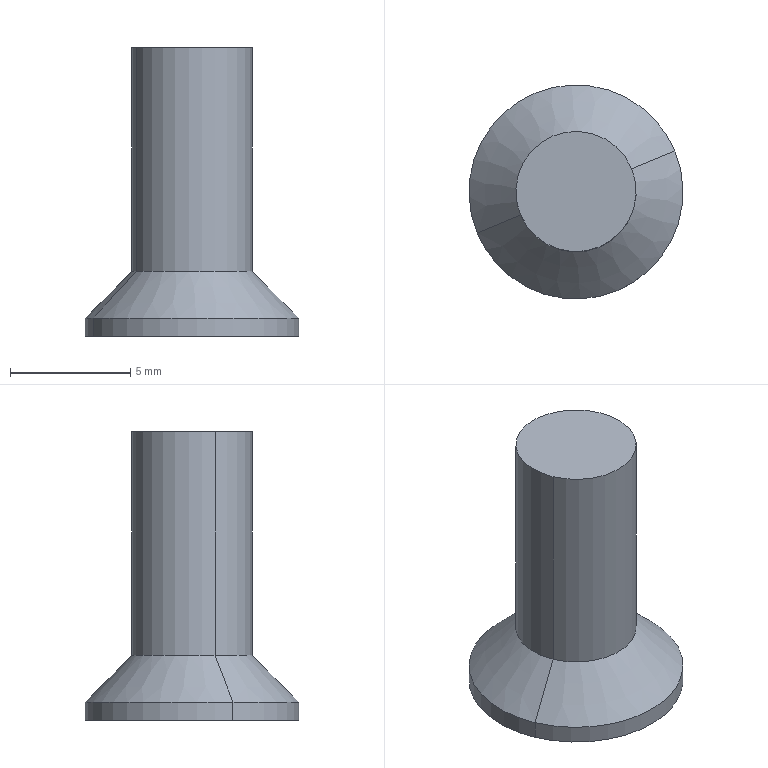Part | SolidWorks | features SplitBody 1 | 1 solid | 41 faces | box 8.9 x 8.9 x 12 mm | volume 292.842 mm3 | plane 31 | cylinder 8 | cone 2 | commonest cylinder face diameters 0.6 x4 5 x2 8.9 x2
STEP:
#1=CARTESIAN_POINT('',(595.745,101.287,-497.016));
#2=VERTEX_POINT('',#1);
#3=CARTESIAN_POINT('',(591.126,99.372,-497.016));
#4=VERTEX_POINT('',#3);
#5=CARTESIAN_POINT('',(593.436,100.329,-497.016));
#6=DIRECTION('',(0.,0.,1.));
#7=DIRECTION('',(0.9237,0.383,0.));
#8=AXIS2_PLACEMENT_3D('',#5,#6,#7);
#9=CIRCLE('',#8,2.5);
#10=EDGE_CURVE('',#2,#4,#9,.T.);
#11=ORIENTED_EDGE('',*,*,#10,.T.);
#12=CARTESIAN_POINT('',(591.126,99.372,-487.716));
#13=VERTEX_POINT('',#12);
#14=CARTESIAN_POINT('',(591.126,99.372,-495.2));
#15=DIRECTION('',(0.,0.,1.));
#16=VECTOR('',#15,1000.);
#17=LINE('',#14,#16);
#18=EDGE_CURVE('',#4,#13,#17,.T.);
#19=ORIENTED_EDGE('',*,*,#18,.T.);
#20=CARTESIAN_POINT('',(595.745,101.287,-487.716));
#21=VERTEX_POINT('',#20);
#22=CARTESIAN_POINT('',(593.436,100.329,-487.716));
#23=DIRECTION('',(0.,0.,1.));
#24=DIRECTION('',(0.9237,0.383,0.));
#25=AXIS2_PLACEMENT_3D('',#22,#23,#24);
#26=CIRCLE('',#25,2.5);
#27=EDGE_CURVE('',#21,#13,#26,.T.);
#28=ORIENTED_EDGE('',*,*,#27,.F.);
#29=CARTESIAN_POINT('',(595.745,101.287,-495.2));
#30=DIRECTION('',(0.,0.,1.));
#31=VECTOR('',#30,1000.);
#32=LINE('',#29,#31);
#33=EDGE_CURVE('',#2,#21,#32,.T.);
#34=ORIENTED_EDGE('',*,*,#33,.F.);
#35=EDGE_LOOP('',(#11,#19,#28,#34));
#36=FACE_OUTER_BOUND('',#35,.T.);
#37=CARTESIAN_POINT('',(593.436,100.329,-495.2));
#38=DIRECTION('',(0.,0.,1.));
#39=DIRECTION('',(0.9237,0.383,0.));
#40=AXIS2_PLACEMENT_3D('',#37,#38,#39);
#41=CYLINDRICAL_SURFACE('',#40,2.5);
#42=ADVANCED_FACE('',(#36),#41,.T.);
#43=ORIENTED_EDGE('',*,*,#10,.F.);
#44=CARTESIAN_POINT('',(597.546,102.034,-498.966));
#45=VERTEX_POINT('',#44);
#46=CARTESIAN_POINT('',(595.745,101.287,-497.016));
#47=DIRECTION('',(0.6532,0.2709,-0.7071));
#48=VECTOR('',#47,1000.);
#49=LINE('',#46,#48);
#50=EDGE_CURVE('',#2,#45,#49,.T.);
#51=ORIENTED_EDGE('',*,*,#50,.T.);
#52=CARTESIAN_POINT('',(589.325,98.625,-498.966));
#53=VERTEX_POINT('',#52);
#54=CARTESIAN_POINT('',(593.436,100.329,-498.966));
#55=DIRECTION('',(0.,0.,1.));
#56=DIRECTION('',(0.9237,0.383,0.));
#57=AXIS2_PLACEMENT_3D('',#54,#55,#56);
#58=CIRCLE('',#57,4.45);
#59=EDGE_CURVE('',#45,#53,#58,.T.);
#60=ORIENTED_EDGE('',*,*,#59,.T.);
#61=CARTESIAN_POINT('',(591.126,99.372,-497.016));
#62=DIRECTION('',(-0.6532,-0.2709,-0.7071));
#63=VECTOR('',#62,1000.);
#64=LINE('',#61,#63);
#65=EDGE_CURVE('',#4,#53,#64,.T.);
#66=ORIENTED_EDGE('',*,*,#65,.F.);
#67=EDGE_LOOP('',(#43,#51,#60,#66));
#68=FACE_OUTER_BOUND('',#67,.T.);
#69=CARTESIAN_POINT('',(593.436,100.329,-497.016));
#70=DIRECTION('',(0.,0.,-1.));
#71=DIRECTION('',(-0.9237,-0.383,0.));
#72=AXIS2_PLACEMENT_3D('',#69,#70,#71);
#73=CONICAL_SURFACE('',#72,2.5,0.7854);
#74=ADVANCED_FACE('',(#68),#73,.T.);
#75=CARTESIAN_POINT('',(597.546,102.034,-499.716));
#76=VERTEX_POINT('',#75);
#77=CARTESIAN_POINT('',(589.325,98.625,-499.716));
#78=VERTEX_POINT('',#77);
#79=CARTESIAN_POINT('',(593.436,100.329,-499.716));
#80=DIRECTION('',(0.,0.,1.));
#81=DIRECTION('',(0.9237,0.383,0.));
#82=AXIS2_PLACEMENT_3D('',#79,#80,#81);
#83=CIRCLE('',#82,4.45);
#84=EDGE_CURVE('',#76,#78,#83,.T.);
#85=ORIENTED_EDGE('',*,*,#84,.T.);
#86=CARTESIAN_POINT('',(589.325,98.625,-495.2));
#87=DIRECTION('',(0.,0.,1.));
#88=VECTOR('',#87,1000.);
#89=LINE('',#86,#88);
#90=EDGE_CURVE('',#78,#53,#89,.T.);
#91=ORIENTED_EDGE('',*,*,#90,.T.);
#92=ORIENTED_EDGE('',*,*,#59,.F.);
#93=CARTESIAN_POINT('',(597.546,102.034,-495.2));
#94=DIRECTION('',(0.,0.,1.));
#95=VECTOR('',#94,1000.);
#96=LINE('',#93,#95);
#97=EDGE_CURVE('',#76,#45,#96,.T.);
#98=ORIENTED_EDGE('',*,*,#97,.F.);
#99=EDGE_LOOP('',(#85,#91,#92,#98));
#100=FACE_OUTER_BOUND('',#99,.T.);
#101=CARTESIAN_POINT('',(593.436,100.329,-495.2));
#102=DIRECTION('',(0.,0.,1.));
#103=DIRECTION('',(0.9237,0.383,0.));
#104=AXIS2_PLACEMENT_3D('',#101,#102,#103);
#105=CYLINDRICAL_SURFACE('',#104,4.45);
#106=ADVANCED_FACE('',(#100),#105,.T.);
#107=ORIENTED_EDGE('',*,*,#84,.F.);
#108=CARTESIAN_POINT('',(593.436,100.329,-499.716));
#109=DIRECTION('',(0.,0.,1.));
#110=DIRECTION('',(0.9237,0.383,0.));
#111=AXIS2_PLACEMENT_3D('',#108,#109,#110);
#112=CIRCLE('',#111,4.45);
#113=EDGE_CURVE('',#78,#76,#112,.T.);
#114=ORIENTED_EDGE('',*,*,#113,.F.);
#115=EDGE_LOOP('',(#107,#114));
#116=FACE_OUTER_BOUND('',#115,.T.);
#117=CARTESIAN_POINT('',(595.638,101.806,-499.716));
#118=VERTEX_POINT('',#117);
#119=CARTESIAN_POINT('',(594.232,101.222,-499.716));
#120=VERTEX_POINT('',#119);
#121=CARTESIAN_POINT('',(593.717,101.009,-499.716));
#122=DIRECTION('',(-0.9237,-0.383,0.));
#123=VECTOR('',#122,1000.);
#124=LINE('',#121,#123);
#125=EDGE_CURVE('',#118,#120,#124,.T.);
#126=ORIENTED_EDGE('',*,*,#125,.T.);
#127=CARTESIAN_POINT('',(594.43,102.732,-499.716));
#128=VERTEX_POINT('',#127);
#129=CARTESIAN_POINT('',(594.153,100.627,-499.716));
#130=DIRECTION('',(0.1301,0.9915,0.));
#131=VECTOR('',#130,1000.);
#132=LINE('',#129,#131);
#133=EDGE_CURVE('',#120,#128,#132,.T.);
#134=ORIENTED_EDGE('',*,*,#133,.T.);
#135=CARTESIAN_POINT('',(593.503,101.524,-499.716));
#136=VERTEX_POINT('',#135);
#137=CARTESIAN_POINT('',(593.138,101.047,-499.716));
#138=DIRECTION('',(-0.6084,-0.7936,0.));
#139=VECTOR('',#138,1000.);
#140=LINE('',#137,#139);
#141=EDGE_CURVE('',#128,#136,#140,.T.);
#142=ORIENTED_EDGE('',*,*,#141,.T.);
#143=CARTESIAN_POINT('',(592.92,102.93,-499.716));
#144=VERTEX_POINT('',#143);
#145=CARTESIAN_POINT('',(593.717,101.009,-499.716));
#146=DIRECTION('',(-0.383,0.9237,0.));
#147=VECTOR('',#146,1000.);
#148=LINE('',#145,#147);
#149=EDGE_CURVE('',#136,#144,#148,.T.);
#150=ORIENTED_EDGE('',*,*,#149,.T.);
#151=CARTESIAN_POINT('',(591.959,102.532,-499.716));
#152=VERTEX_POINT('',#151);
#153=CARTESIAN_POINT('',(592.92,102.93,-499.716));
#154=DIRECTION('',(-0.9237,-0.383,0.));
#155=VECTOR('',#154,1000.);
#156=LINE('',#153,#155);
#157=EDGE_CURVE('',#144,#152,#156,.T.);
#158=ORIENTED_EDGE('',*,*,#157,.T.);
#159=CARTESIAN_POINT('',(592.543,101.125,-499.716));
#160=VERTEX_POINT('',#159);
#161=CARTESIAN_POINT('',(592.756,100.611,-499.716));
#162=DIRECTION('',(0.383,-0.9237,0.));
#163=VECTOR('',#162,1000.);
#164=LINE('',#161,#163);
#165=EDGE_CURVE('',#152,#160,#164,.T.);
#166=ORIENTED_EDGE('',*,*,#165,.T.);
#167=CARTESIAN_POINT('',(591.033,101.323,-499.716));
#168=VERTEX_POINT('',#167);
#169=CARTESIAN_POINT('',(593.138,101.047,-499.716));
#170=DIRECTION('',(-0.9915,0.1301,0.));
#171=VECTOR('',#170,1000.);
#172=LINE('',#169,#171);
#173=EDGE_CURVE('',#160,#168,#172,.T.);
#174=ORIENTED_EDGE('',*,*,#173,.T.);
#175=CARTESIAN_POINT('',(592.241,100.397,-499.716));
#176=VERTEX_POINT('',#175);
#177=CARTESIAN_POINT('',(592.718,100.032,-499.716));
#178=DIRECTION('',(0.7936,-0.6084,0.));
#179=VECTOR('',#178,1000.);
#180=LINE('',#177,#179);
#181=EDGE_CURVE('',#168,#176,#180,.T.);
#182=ORIENTED_EDGE('',*,*,#181,.T.);
#183=CARTESIAN_POINT('',(590.835,99.814,-499.716));
#184=VERTEX_POINT('',#183);
#185=CARTESIAN_POINT('',(592.756,100.611,-499.716));
#186=DIRECTION('',(-0.9237,-0.383,0.));
#187=VECTOR('',#186,1000.);
#188=LINE('',#185,#187);
#189=EDGE_CURVE('',#176,#184,#188,.T.);
#190=ORIENTED_EDGE('',*,*,#189,.T.);
#191=CARTESIAN_POINT('',(591.233,98.853,-499.716));
#192=VERTEX_POINT('',#191);
#193=CARTESIAN_POINT('',(590.835,99.814,-499.716));
#194=DIRECTION('',(0.383,-0.9237,0.));
#195=VECTOR('',#194,1000.);
#196=LINE('',#193,#195);
#197=EDGE_CURVE('',#184,#192,#196,.T.);
#198=ORIENTED_EDGE('',*,*,#197,.T.);
#199=CARTESIAN_POINT('',(592.64,99.436,-499.716));
#200=VERTEX_POINT('',#199);
#201=CARTESIAN_POINT('',(593.155,99.65,-499.716));
#202=DIRECTION('',(0.9237,0.383,0.));
#203=VECTOR('',#202,1000.);
#204=LINE('',#201,#203);
#205=EDGE_CURVE('',#192,#200,#204,.T.);
#206=ORIENTED_EDGE('',*,*,#205,.T.);
#207=CARTESIAN_POINT('',(592.442,97.927,-499.716));
#208=VERTEX_POINT('',#207);
#209=CARTESIAN_POINT('',(592.718,100.032,-499.716));
#210=DIRECTION('',(-0.1301,-0.9915,0.));
#211=VECTOR('',#210,1000.);
#212=LINE('',#209,#211);
#213=EDGE_CURVE('',#200,#208,#212,.T.);
#214=ORIENTED_EDGE('',*,*,#213,.T.);
#215=CARTESIAN_POINT('',(593.368,99.135,-499.716));
#216=VERTEX_POINT('',#215);
#217=CARTESIAN_POINT('',(593.733,99.612,-499.716));
#218=DIRECTION('',(0.6084,0.7936,0.));
#219=VECTOR('',#218,1000.);
#220=LINE('',#217,#219);
#221=EDGE_CURVE('',#208,#216,#220,.T.);
#222=ORIENTED_EDGE('',*,*,#221,.T.);
#223=CARTESIAN_POINT('',(593.951,97.728,-499.716));
#224=VERTEX_POINT('',#223);
#225=CARTESIAN_POINT('',(593.155,99.65,-499.716));
#226=DIRECTION('',(0.383,-0.9237,0.));
#227=VECTOR('',#226,1000.);
#228=LINE('',#225,#227);
#229=EDGE_CURVE('',#216,#224,#228,.T.);
#230=ORIENTED_EDGE('',*,*,#229,.T.);
#231=CARTESIAN_POINT('',(594.912,98.127,-499.716));
#232=VERTEX_POINT('',#231);
#233=CARTESIAN_POINT('',(594.912,98.127,-499.716));
#234=DIRECTION('',(0.9237,0.383,0.));
#235=VECTOR('',#234,1000.);
#236=LINE('',#233,#235);
#237=EDGE_CURVE('',#224,#232,#236,.T.);
#238=ORIENTED_EDGE('',*,*,#237,.T.);
#239=CARTESIAN_POINT('',(594.329,99.533,-499.716));
#240=VERTEX_POINT('',#239);
#241=CARTESIAN_POINT('',(594.115,100.048,-499.716));
#242=DIRECTION('',(-0.383,0.9237,0.));
#243=VECTOR('',#242,1000.);
#244=LINE('',#241,#243);
#245=EDGE_CURVE('',#232,#240,#244,.T.);
#246=ORIENTED_EDGE('',*,*,#245,.T.);
#247=CARTESIAN_POINT('',(595.838,99.335,-499.716));
#248=VERTEX_POINT('',#247);
#249=CARTESIAN_POINT('',(593.733,99.612,-499.716));
#250=DIRECTION('',(0.9915,-0.1301,0.));
#251=VECTOR('',#250,1000.);
#252=LINE('',#249,#251);
#253=EDGE_CURVE('',#240,#248,#252,.T.);
#254=ORIENTED_EDGE('',*,*,#253,.T.);
#255=CARTESIAN_POINT('',(594.63,100.262,-499.716));
#256=VERTEX_POINT('',#255);
#257=CARTESIAN_POINT('',(594.153,100.627,-499.716));
#258=DIRECTION('',(-0.7936,0.6084,0.));
#259=VECTOR('',#258,1000.);
#260=LINE('',#257,#259);
#261=EDGE_CURVE('',#248,#256,#260,.T.);
#262=ORIENTED_EDGE('',*,*,#261,.T.);
#263=CARTESIAN_POINT('',(596.037,100.845,-499.716));
#264=VERTEX_POINT('',#263);
#265=CARTESIAN_POINT('',(594.115,100.048,-499.716));
#266=DIRECTION('',(0.9237,0.383,0.));
#267=VECTOR('',#266,1000.);
#268=LINE('',#265,#267);
#269=EDGE_CURVE('',#256,#264,#268,.T.);
#270=ORIENTED_EDGE('',*,*,#269,.T.);
#271=CARTESIAN_POINT('',(595.638,101.806,-499.716));
#272=DIRECTION('',(-0.383,0.9237,0.));
#273=VECTOR('',#272,1000.);
#274=LINE('',#271,#273);
#275=EDGE_CURVE('',#264,#118,#274,.T.);
#276=ORIENTED_EDGE('',*,*,#275,.T.);
#277=EDGE_LOOP('',(#126,#134,#142,#150,#158,#166,#174,#182,#190,#198,#206,#214,#222,#230,#238,#246,#254,#262,#270,#276));
#278=FACE_BOUND('',#277,.T.);
#279=CARTESIAN_POINT('',(591.731,104.44,-499.716));
#280=DIRECTION('',(0.,0.,-1.));
#281=DIRECTION('',(-0.9237,-0.383,0.));
#282=AXIS2_PLACEMENT_3D('',#279,#280,#281);
#283=PLANE('',#282);
#284=ADVANCED_FACE('',(#116,#278),#283,.T.);
#285=ORIENTED_EDGE('',*,*,#189,.F.);
#286=CARTESIAN_POINT('',(592.479,100.496,-499.104));
#287=VERTEX_POINT('',#286);
#288=CARTESIAN_POINT('',(592.764,100.614,-498.37));
#289=DIRECTION('',(0.3579,0.1484,0.9219));
#290=VECTOR('',#289,1000.);
#291=LINE('',#288,#290);
#292=EDGE_CURVE('',#176,#287,#291,.T.);
#293=ORIENTED_EDGE('',*,*,#292,.T.);
#294=CARTESIAN_POINT('',(592.479,100.496,-498.366));
#295=VERTEX_POINT('',#294);
#296=CARTESIAN_POINT('',(592.479,100.496,-498.366));
#297=DIRECTION('',(0.,0.,1.));
#298=VECTOR('',#297,1000.);
#299=LINE('',#296,#298);
#300=EDGE_CURVE('',#287,#295,#299,.T.);
#301=ORIENTED_EDGE('',*,*,#300,.T.);
#302=CARTESIAN_POINT('',(591.555,100.112,-498.366));
#303=VERTEX_POINT('',#302);
#304=CARTESIAN_POINT('',(592.756,100.611,-498.366));
#305=DIRECTION('',(-0.9237,-0.383,0.));
#306=VECTOR('',#305,1000.);
#307=LINE('',#304,#306);
#308=EDGE_CURVE('',#295,#303,#307,.T.);
#309=ORIENTED_EDGE('',*,*,#308,.T.);
#310=CARTESIAN_POINT('',(590.835,99.814,-499.716));
#311=DIRECTION('',(-0.4619,-0.1915,-0.866));
#312=VECTOR('',#311,1000.);
#313=LINE('',#310,#312);
#314=EDGE_CURVE('',#303,#184,#313,.T.);
#315=ORIENTED_EDGE('',*,*,#314,.T.);
#316=EDGE_LOOP('',(#285,#293,#301,#309,#315));
#317=FACE_OUTER_BOUND('',#316,.T.);
#318=CARTESIAN_POINT('',(592.756,100.611,-498.366));
#319=DIRECTION('',(0.383,-0.9237,0.));
#320=DIRECTION('',(0.9237,0.383,0.));
#321=AXIS2_PLACEMENT_3D('',#318,#319,#320);
#322=PLANE('',#321);
#323=ADVANCED_FACE('',(#317),#322,.T.);
#324=CARTESIAN_POINT('',(592.877,99.535,-498.366));
#325=VERTEX_POINT('',#324);
#326=CARTESIAN_POINT('',(592.877,99.535,-499.104));
#327=VERTEX_POINT('',#326);
#328=CARTESIAN_POINT('',(592.877,99.535,-498.366));
#329=DIRECTION('',(0.,0.,-1.));
#330=VECTOR('',#329,1000.);
#331=LINE('',#328,#330);
#332=EDGE_CURVE('',#325,#327,#331,.T.);
#333=ORIENTED_EDGE('',*,*,#332,.T.);
#334=CARTESIAN_POINT('',(593.162,99.653,-498.37));
#335=DIRECTION('',(-0.3579,-0.1484,-0.9219));
#336=VECTOR('',#335,1000.);
#337=LINE('',#334,#336);
#338=EDGE_CURVE('',#327,#200,#337,.T.);
#339=ORIENTED_EDGE('',*,*,#338,.T.);
#340=ORIENTED_EDGE('',*,*,#205,.F.);
#341=CARTESIAN_POINT('',(591.953,99.152,-498.366));
#342=VERTEX_POINT('',#341);
#343=CARTESIAN_POINT('',(592.254,99.276,-497.803));
#344=DIRECTION('',(-0.4619,-0.1915,-0.866));
#345=VECTOR('',#344,1000.);
#346=LINE('',#343,#345);
#347=EDGE_CURVE('',#342,#192,#346,.T.);
#348=ORIENTED_EDGE('',*,*,#347,.F.);
#349=CARTESIAN_POINT('',(593.155,99.65,-498.366));
#350=DIRECTION('',(0.9237,0.383,0.));
#351=VECTOR('',#350,1000.);
#352=LINE('',#349,#351);
#353=EDGE_CURVE('',#342,#325,#352,.T.);
#354=ORIENTED_EDGE('',*,*,#353,.T.);
#355=EDGE_LOOP('',(#333,#339,#340,#348,#354));
#356=FACE_OUTER_BOUND('',#355,.T.);
#357=CARTESIAN_POINT('',(593.155,99.65,-498.366));
#358=DIRECTION('',(-0.383,0.9237,0.));
#359=DIRECTION('',(-0.9237,-0.383,0.));
#360=AXIS2_PLACEMENT_3D('',#357,#358,#359);
#361=PLANE('',#360);
#362=ADVANCED_FACE('',(#356),#361,.T.);
#363=ORIENTED_EDGE('',*,*,#229,.F.);
#364=CARTESIAN_POINT('',(593.269,99.373,-499.104));
#365=VERTEX_POINT('',#364);
#366=CARTESIAN_POINT('',(593.151,99.658,-498.37));
#367=DIRECTION('',(-0.1484,0.3579,0.9219));
#368=VECTOR('',#367,1000.);
#369=LINE('',#366,#368);
#370=EDGE_CURVE('',#216,#365,#369,.T.);
#371=ORIENTED_EDGE('',*,*,#370,.T.);
#372=CARTESIAN_POINT('',(593.269,99.373,-498.366));
#373=VERTEX_POINT('',#372);
#374=CARTESIAN_POINT('',(593.269,99.373,-498.366));
#375=DIRECTION('',(0.,0.,1.));
#376=VECTOR('',#375,1000.);
#377=LINE('',#374,#376);
#378=EDGE_CURVE('',#365,#373,#377,.T.);
#379=ORIENTED_EDGE('',*,*,#378,.T.);
#380=CARTESIAN_POINT('',(593.653,98.448,-498.366));
#381=VERTEX_POINT('',#380);
#382=CARTESIAN_POINT('',(593.155,99.65,-498.366));
#383=DIRECTION('',(0.383,-0.9237,0.));
#384=VECTOR('',#383,1000.);
#385=LINE('',#382,#384);
#386=EDGE_CURVE('',#373,#381,#385,.T.);
#387=ORIENTED_EDGE('',*,*,#386,.T.);
#388=CARTESIAN_POINT('',(593.951,97.728,-499.716));
#389=DIRECTION('',(0.1915,-0.4619,-0.866));
#390=VECTOR('',#389,1000.);
#391=LINE('',#388,#390);
#392=EDGE_CURVE('',#381,#224,#391,.T.);
#393=ORIENTED_EDGE('',*,*,#392,.T.);
#394=EDGE_LOOP('',(#363,#371,#379,#387,#393));
#395=FACE_OUTER_BOUND('',#394,.T.);
#396=CARTESIAN_POINT('',(593.155,99.65,-498.366));
#397=DIRECTION('',(0.9237,0.383,0.));
#398=DIRECTION('',(-0.383,0.9237,0.));
#399=AXIS2_PLACEMENT_3D('',#396,#397,#398);
#400=PLANE('',#399);
#401=ADVANCED_FACE('',(#395),#400,.T.);
#402=CARTESIAN_POINT('',(594.23,99.771,-498.366));
#403=VERTEX_POINT('',#402);
#404=CARTESIAN_POINT('',(594.23,99.771,-499.104));
#405=VERTEX_POINT('',#404);
#406=CARTESIAN_POINT('',(594.23,99.771,-498.366));
#407=DIRECTION('',(0.,0.,-1.));
#408=VECTOR('',#407,1000.);
#409=LINE('',#406,#408);
#410=EDGE_CURVE('',#403,#405,#409,.T.);
#411=ORIENTED_EDGE('',*,*,#410,.T.);
#412=CARTESIAN_POINT('',(594.112,100.056,-498.37));
#413=DIRECTION('',(0.1484,-0.3579,-0.9219));
#414=VECTOR('',#413,1000.);
#415=LINE('',#412,#414);
#416=EDGE_CURVE('',#405,#240,#415,.T.);
#417=ORIENTED_EDGE('',*,*,#416,.T.);
#418=ORIENTED_EDGE('',*,*,#245,.F.);
#419=CARTESIAN_POINT('',(594.613,98.847,-498.366));
#420=VERTEX_POINT('',#419);
#421=CARTESIAN_POINT('',(594.489,99.147,-497.803));
#422=DIRECTION('',(0.1915,-0.4619,-0.866));
#423=VECTOR('',#422,1000.);
#424=LINE('',#421,#423);
#425=EDGE_CURVE('',#420,#232,#424,.T.);
#426=ORIENTED_EDGE('',*,*,#425,.F.);
#427=CARTESIAN_POINT('',(594.115,100.048,-498.366));
#428=DIRECTION('',(-0.383,0.9237,0.));
#429=VECTOR('',#428,1000.);
#430=LINE('',#427,#429);
#431=EDGE_CURVE('',#420,#403,#430,.T.);
#432=ORIENTED_EDGE('',*,*,#431,.T.);
#433=EDGE_LOOP('',(#411,#417,#418,#426,#432));
#434=FACE_OUTER_BOUND('',#433,.T.);
#435=CARTESIAN_POINT('',(594.115,100.048,-498.366));
#436=DIRECTION('',(-0.9237,-0.383,0.));
#437=DIRECTION('',(0.,0.,1.));
#438=AXIS2_PLACEMENT_3D('',#435,#436,#437);
#439=PLANE('',#438);
#440=ADVANCED_FACE('',(#434),#439,.T.);
#441=ORIENTED_EDGE('',*,*,#269,.F.);
#442=CARTESIAN_POINT('',(594.392,100.163,-499.104));
#443=VERTEX_POINT('',#442);
#444=CARTESIAN_POINT('',(594.107,100.045,-498.37));
#445=DIRECTION('',(-0.3579,-0.1484,0.9219));
#446=VECTOR('',#445,1000.);
#447=LINE('',#444,#446);
#448=EDGE_CURVE('',#256,#443,#447,.T.);
#449=ORIENTED_EDGE('',*,*,#448,.T.);
#450=CARTESIAN_POINT('',(594.392,100.163,-498.366));
#451=VERTEX_POINT('',#450);
#452=CARTESIAN_POINT('',(594.392,100.163,-498.366));
#453=DIRECTION('',(0.,0.,1.));
#454=VECTOR('',#453,1000.);
#455=LINE('',#452,#454);
#456=EDGE_CURVE('',#443,#451,#455,.T.);
#457=ORIENTED_EDGE('',*,*,#456,.T.);
#458=CARTESIAN_POINT('',(595.317,100.546,-498.366));
#459=VERTEX_POINT('',#458);
#460=CARTESIAN_POINT('',(594.115,100.048,-498.366));
#461=DIRECTION('',(0.9237,0.383,0.));
#462=VECTOR('',#461,1000.);
#463=LINE('',#460,#462);
#464=EDGE_CURVE('',#451,#459,#463,.T.);
#465=ORIENTED_EDGE('',*,*,#464,.T.);
#466=CARTESIAN_POINT('',(596.037,100.845,-499.716));
#467=DIRECTION('',(0.4619,0.1915,-0.866));
#468=VECTOR('',#467,1000.);
#469=LINE('',#466,#468);
#470=EDGE_CURVE('',#459,#264,#469,.T.);
#471=ORIENTED_EDGE('',*,*,#470,.T.);
#472=EDGE_LOOP('',(#441,#449,#457,#465,#471));
#473=FACE_OUTER_BOUND('',#472,.T.);
#474=CARTESIAN_POINT('',(594.115,100.048,-498.366));
#475=DIRECTION('',(-0.383,0.9237,0.));
#476=DIRECTION('',(-0.9237,-0.383,0.));
#477=AXIS2_PLACEMENT_3D('',#474,#475,#476);
#478=PLANE('',#477);
#479=ADVANCED_FACE('',(#473),#478,.T.);
#480=CARTESIAN_POINT('',(593.994,101.124,-498.366));
#481=VERTEX_POINT('',#480);
#482=CARTESIAN_POINT('',(593.994,101.124,-499.104));
#483=VERTEX_POINT('',#482);
#484=CARTESIAN_POINT('',(593.994,101.124,-498.366));
#485=DIRECTION('',(0.,0.,-1.));
#486=VECTOR('',#485,1000.);
#487=LINE('',#484,#486);
#488=EDGE_CURVE('',#481,#483,#487,.T.);
#489=ORIENTED_EDGE('',*,*,#488,.T.);
#490=CARTESIAN_POINT('',(593.709,101.006,-498.37));
#491=DIRECTION('',(0.3579,0.1484,-0.9219));
#492=VECTOR('',#491,1000.);
#493=LINE('',#490,#492);
#494=EDGE_CURVE('',#483,#120,#493,.T.);
#495=ORIENTED_EDGE('',*,*,#494,.T.);
#496=ORIENTED_EDGE('',*,*,#125,.F.);
#497=CARTESIAN_POINT('',(594.918,101.507,-498.366));
#498=VERTEX_POINT('',#497);
#499=CARTESIAN_POINT('',(594.618,101.383,-497.803));
#500=DIRECTION('',(0.4619,0.1915,-0.866));
#501=VECTOR('',#500,1000.);
#502=LINE('',#499,#501);
#503=EDGE_CURVE('',#498,#118,#502,.T.);
#504=ORIENTED_EDGE('',*,*,#503,.F.);
#505=CARTESIAN_POINT('',(593.717,101.009,-498.366));
#506=DIRECTION('',(-0.9237,-0.383,0.));
#507=VECTOR('',#506,1000.);
#508=LINE('',#505,#507);
#509=EDGE_CURVE('',#498,#481,#508,.T.);
#510=ORIENTED_EDGE('',*,*,#509,.T.);
#511=EDGE_LOOP('',(#489,#495,#496,#504,#510));
#512=FACE_OUTER_BOUND('',#511,.T.);
#513=CARTESIAN_POINT('',(593.717,101.009,-498.366));
#514=DIRECTION('',(0.383,-0.9237,0.));
#515=DIRECTION('',(0.9237,0.383,0.));
#516=AXIS2_PLACEMENT_3D('',#513,#514,#515);
#517=PLANE('',#516);
#518=ADVANCED_FACE('',(#512),#517,.T.);
#519=ORIENTED_EDGE('',*,*,#149,.F.);
#520=CARTESIAN_POINT('',(593.602,101.286,-499.104));
#521=VERTEX_POINT('',#520);
#522=CARTESIAN_POINT('',(593.72,101.001,-498.37));
#523=DIRECTION('',(0.1484,-0.3579,0.9219));
#524=VECTOR('',#523,1000.);
#525=LINE('',#522,#524);
#526=EDGE_CURVE('',#136,#521,#525,.T.);
#527=ORIENTED_EDGE('',*,*,#526,.T.);
#528=CARTESIAN_POINT('',(593.602,101.286,-498.366));
#529=VERTEX_POINT('',#528);
#530=CARTESIAN_POINT('',(593.602,101.286,-498.366));
#531=DIRECTION('',(0.,0.,1.));
#532=VECTOR('',#531,1000.);
#533=LINE('',#530,#532);
#534=EDGE_CURVE('',#521,#529,#533,.T.);
#535=ORIENTED_EDGE('',*,*,#534,.T.);
#536=CARTESIAN_POINT('',(593.219,102.21,-498.366));
#537=VERTEX_POINT('',#536);
#538=CARTESIAN_POINT('',(593.717,101.009,-498.366));
#539=DIRECTION('',(-0.383,0.9237,0.));
#540=VECTOR('',#539,1000.);
#541=LINE('',#538,#540);
#542=EDGE_CURVE('',#529,#537,#541,.T.);
#543=ORIENTED_EDGE('',*,*,#542,.T.);
#544=CARTESIAN_POINT('',(592.92,102.93,-499.716));
#545=DIRECTION('',(-0.1915,0.4619,-0.866));
#546=VECTOR('',#545,1000.);
#547=LINE('',#544,#546);
#548=EDGE_CURVE('',#537,#144,#547,.T.);
#549=ORIENTED_EDGE('',*,*,#548,.T.);
#550=EDGE_LOOP('',(#519,#527,#535,#543,#549));
#551=FACE_OUTER_BOUND('',#550,.T.);
#552=CARTESIAN_POINT('',(593.717,101.009,-498.366));
#553=DIRECTION('',(-0.9237,-0.383,0.));
#554=DIRECTION('',(0.,0.,1.));
#555=AXIS2_PLACEMENT_3D('',#552,#553,#554);
#556=PLANE('',#555);
#557=ADVANCED_FACE('',(#551),#556,.T.);
#558=CARTESIAN_POINT('',(592.641,100.888,-498.366));
#559=VERTEX_POINT('',#558);
#560=CARTESIAN_POINT('',(592.641,100.888,-499.104));
#561=VERTEX_POINT('',#560);
#562=CARTESIAN_POINT('',(592.641,100.888,-498.366));
#563=DIRECTION('',(0.,0.,-1.));
#564=VECTOR('',#563,1000.);
#565=LINE('',#562,#564);
#566=EDGE_CURVE('',#559,#561,#565,.T.);
#567=ORIENTED_EDGE('',*,*,#566,.T.);
#568=CARTESIAN_POINT('',(592.759,100.603,-498.37));
#569=DIRECTION('',(-0.1484,0.3579,-0.9219));
#570=VECTOR('',#569,1000.);
#571=LINE('',#568,#570);
#572=EDGE_CURVE('',#561,#160,#571,.T.);
#573=ORIENTED_EDGE('',*,*,#572,.T.);
#574=ORIENTED_EDGE('',*,*,#165,.F.);
#575=CARTESIAN_POINT('',(592.258,101.812,-498.366));
#576=VERTEX_POINT('',#575);
#577=CARTESIAN_POINT('',(592.383,101.512,-497.803));
#578=DIRECTION('',(-0.1915,0.4619,-0.866));
#579=VECTOR('',#578,1000.);
#580=LINE('',#577,#579);
#581=EDGE_CURVE('',#576,#152,#580,.T.);
#582=ORIENTED_EDGE('',*,*,#581,.F.);
#583=CARTESIAN_POINT('',(592.756,100.611,-498.366));
#584=DIRECTION('',(0.383,-0.9237,0.));
#585=VECTOR('',#584,1000.);
#586=LINE('',#583,#585);
#587=EDGE_CURVE('',#576,#559,#586,.T.);
#588=ORIENTED_EDGE('',*,*,#587,.T.);
#589=EDGE_LOOP('',(#567,#573,#574,#582,#588));
#590=FACE_OUTER_BOUND('',#589,.T.);
#591=CARTESIAN_POINT('',(592.756,100.611,-498.366));
#592=DIRECTION('',(0.9237,0.383,0.));
#593=DIRECTION('',(-0.383,0.9237,0.));
#594=AXIS2_PLACEMENT_3D('',#591,#592,#593);
#595=PLANE('',#594);
#596=ADVANCED_FACE('',(#590),#595,.T.);
#597=ORIENTED_EDGE('',*,*,#308,.F.);
#598=CARTESIAN_POINT('',(592.364,100.773,-498.366));
#599=DIRECTION('',(0.,0.,1.));
#600=DIRECTION('',(0.9237,0.383,0.));
#601=AXIS2_PLACEMENT_3D('',#598,#599,#600);
#602=CIRCLE('',#601,0.3);
#603=EDGE_CURVE('',#295,#559,#602,.T.);
#604=ORIENTED_EDGE('',*,*,#603,.T.);
#605=ORIENTED_EDGE('',*,*,#587,.F.);
#606=CARTESIAN_POINT('',(593.219,102.21,-498.366));
#607=DIRECTION('',(-0.9237,-0.383,0.));
#608=VECTOR('',#607,1000.);
#609=LINE('',#606,#608);
#610=EDGE_CURVE('',#537,#576,#609,.T.);
#611=ORIENTED_EDGE('',*,*,#610,.F.);
#612=ORIENTED_EDGE('',*,*,#542,.F.);
#613=CARTESIAN_POINT('',(593.879,101.401,-498.366));
#614=DIRECTION('',(0.,0.,1.));
#615=DIRECTION('',(0.9237,0.383,0.));
#616=AXIS2_PLACEMENT_3D('',#613,#614,#615);
#617=CIRCLE('',#616,0.3);
#618=EDGE_CURVE('',#529,#481,#617,.T.);
#619=ORIENTED_EDGE('',*,*,#618,.T.);
#620=ORIENTED_EDGE('',*,*,#509,.F.);
#621=CARTESIAN_POINT('',(594.918,101.507,-498.366));
#622=DIRECTION('',(-0.383,0.9237,0.));
#623=VECTOR('',#622,1000.);
#624=LINE('',#621,#623);
#625=EDGE_CURVE('',#459,#498,#624,.T.);
#626=ORIENTED_EDGE('',*,*,#625,.F.);
#627=ORIENTED_EDGE('',*,*,#464,.F.);
#628=CARTESIAN_POINT('',(594.507,99.886,-498.366));
#629=DIRECTION('',(0.,0.,1.));
#630=DIRECTION('',(0.9237,0.383,0.));
#631=AXIS2_PLACEMENT_3D('',#628,#629,#630);
#632=CIRCLE('',#631,0.3);
#633=EDGE_CURVE('',#451,#403,#632,.T.);
#634=ORIENTED_EDGE('',*,*,#633,.T.);
#635=ORIENTED_EDGE('',*,*,#431,.F.);
#636=CARTESIAN_POINT('',(594.613,98.847,-498.366));
#637=DIRECTION('',(0.9237,0.383,0.));
#638=VECTOR('',#637,1000.);
#639=LINE('',#636,#638);
#640=EDGE_CURVE('',#381,#420,#639,.T.);
#641=ORIENTED_EDGE('',*,*,#640,.F.);
#642=ORIENTED_EDGE('',*,*,#386,.F.);
#643=CARTESIAN_POINT('',(592.992,99.258,-498.366));
#644=DIRECTION('',(0.,0.,1.));
#645=DIRECTION('',(0.9237,0.383,0.));
#646=AXIS2_PLACEMENT_3D('',#643,#644,#645);
#647=CIRCLE('',#646,0.3);
#648=EDGE_CURVE('',#373,#325,#647,.T.);
#649=ORIENTED_EDGE('',*,*,#648,.T.);
#650=ORIENTED_EDGE('',*,*,#353,.F.);
#651=CARTESIAN_POINT('',(591.555,100.112,-498.366));
#652=DIRECTION('',(0.383,-0.9237,0.));
#653=VECTOR('',#652,1000.);
#654=LINE('',#651,#653);
#655=EDGE_CURVE('',#303,#342,#654,.T.);
#656=ORIENTED_EDGE('',*,*,#655,.F.);
#657=EDGE_LOOP('',(#597,#604,#605,#611,#612,#619,#620,#626,#627,#634,#635,#641,#642,#649,#650,#656));
#658=FACE_OUTER_BOUND('',#657,.T.);
#659=CARTESIAN_POINT('',(593.629,100.41,-498.366));
#660=VERTEX_POINT('',#659);
#661=CARTESIAN_POINT('',(594.084,100.061,-498.366));
#662=VERTEX_POINT('',#661);
#663=CARTESIAN_POINT('',(592.982,100.906,-498.366));
#664=DIRECTION('',(0.7936,-0.6084,0.));
#665=VECTOR('',#664,1000.);
#666=LINE('',#663,#665);
#667=EDGE_CURVE('',#660,#662,#666,.T.);
#668=ORIENTED_EDGE('',*,*,#667,.F.);
#669=CARTESIAN_POINT('',(593.704,100.978,-498.366));
#670=VERTEX_POINT('',#669);
#671=CARTESIAN_POINT('',(593.641,100.494,-498.366));
#672=DIRECTION('',(-0.1301,-0.9915,0.));
#673=VECTOR('',#672,1000.);
#674=LINE('',#671,#673);
#675=EDGE_CURVE('',#670,#660,#674,.T.);
#676=ORIENTED_EDGE('',*,*,#675,.F.);
#677=CARTESIAN_POINT('',(593.355,100.523,-498.366));
#678=VERTEX_POINT('',#677);
#679=CARTESIAN_POINT('',(593.176,100.289,-498.366));
#680=DIRECTION('',(0.6084,0.7936,0.));
#681=VECTOR('',#680,1000.);
#682=LINE('',#679,#681);
#683=EDGE_CURVE('',#678,#670,#682,.T.);
#684=ORIENTED_EDGE('',*,*,#683,.F.);
#685=CARTESIAN_POINT('',(592.787,100.598,-498.366));
#686=VERTEX_POINT('',#685);
#687=CARTESIAN_POINT('',(592.755,100.602,-498.366));
#688=DIRECTION('',(0.9915,-0.1301,0.));
#689=VECTOR('',#688,1000.);
#690=LINE('',#687,#689);
#691=EDGE_CURVE('',#686,#678,#690,.T.);
#692=ORIENTED_EDGE('',*,*,#691,.F.);
#693=CARTESIAN_POINT('',(593.242,100.249,-498.366));
#694=VERTEX_POINT('',#693);
#695=CARTESIAN_POINT('',(592.762,100.617,-498.366));
#696=DIRECTION('',(-0.7936,0.6084,0.));
#697=VECTOR('',#696,1000.);
#698=LINE('',#695,#697);
#699=EDGE_CURVE('',#694,#686,#698,.T.);
#700=ORIENTED_EDGE('',*,*,#699,.F.);
#701=CARTESIAN_POINT('',(593.168,99.681,-498.366));
#702=VERTEX_POINT('',#701);
#703=CARTESIAN_POINT('',(593.28,100.542,-498.366));
#704=DIRECTION('',(0.1301,0.9915,0.));
#705=VECTOR('',#704,1000.);
#706=LINE('',#703,#705);
#707=EDGE_CURVE('',#702,#694,#706,.T.);
#708=ORIENTED_EDGE('',*,*,#707,.F.);
#709=CARTESIAN_POINT('',(593.516,100.136,-498.366));
#710=VERTEX_POINT('',#709);
#711=CARTESIAN_POINT('',(593.464,100.068,-498.366));
#712=DIRECTION('',(-0.6084,-0.7936,0.));
#713=VECTOR('',#712,1000.);
#714=LINE('',#711,#713);
#715=EDGE_CURVE('',#710,#702,#714,.T.);
#716=ORIENTED_EDGE('',*,*,#715,.F.);
#717=CARTESIAN_POINT('',(592.708,100.242,-498.366));
#718=DIRECTION('',(-0.9915,0.1301,0.));
#719=VECTOR('',#718,1000.);
#720=LINE('',#717,#719);
#721=EDGE_CURVE('',#662,#710,#720,.T.);
#722=ORIENTED_EDGE('',*,*,#721,.F.);
#723=EDGE_LOOP('',(#668,#676,#684,#692,#700,#708,#716,#722));
#724=FACE_BOUND('',#723,.T.);
#725=CARTESIAN_POINT('',(592.756,100.611,-498.366));
#726=DIRECTION('',(0.,0.,1.));
#727=DIRECTION('',(0.9237,0.383,0.));
#728=AXIS2_PLACEMENT_3D('',#725,#726,#727);
#729=PLANE('',#728);
#730=ADVANCED_FACE('',(#658,#724),#729,.F.);
#731=ORIENTED_EDGE('',*,*,#456,.F.);
#732=CARTESIAN_POINT('',(594.23,100.001,-498.479));
#733=VERTEX_POINT('',#732);
#734=CARTESIAN_POINT('',(594.392,100.163,-499.104));
#735=CARTESIAN_POINT('',(594.318,100.132,-498.912));
#736=CARTESIAN_POINT('',(594.261,100.075,-498.693));
#737=CARTESIAN_POINT('',(594.23,100.001,-498.479));
#738=(BOUNDED_CURVE()B_SPLINE_CURVE(3,(#734,#735,#736,#737),.UNSPECIFIED.,.F.,.T.)B_SPLINE_CURVE_WITH_KNOTS((4,4),(1.047,1.833),.UNSPECIFIED.)CURVE()GEOMETRIC_REPRESENTATION_ITEM()RATIONAL_B_SPLINE_CURVE((1.,0.9493,0.9493,1.))REPRESENTATION_ITEM(''));
#739=EDGE_CURVE('',#443,#733,#738,.T.);
#740=ORIENTED_EDGE('',*,*,#739,.T.);
#741=CARTESIAN_POINT('',(594.23,100.001,-498.479));
#742=CARTESIAN_POINT('',(594.199,99.926,-498.693));
#743=CARTESIAN_POINT('',(594.199,99.846,-498.912));
#744=CARTESIAN_POINT('',(594.23,99.771,-499.104));
#745=(BOUNDED_CURVE()B_SPLINE_CURVE(3,(#741,#742,#743,#744),.UNSPECIFIED.,.F.,.F.)B_SPLINE_CURVE_WITH_KNOTS((4,4),(4.451,5.236),.UNSPECIFIED.)CURVE()GEOMETRIC_REPRESENTATION_ITEM()RATIONAL_B_SPLINE_CURVE((1.,0.9493,0.9493,1.))REPRESENTATION_ITEM(''));
#746=EDGE_CURVE('',#733,#405,#745,.T.);
#747=ORIENTED_EDGE('',*,*,#746,.T.);
#748=ORIENTED_EDGE('',*,*,#410,.F.);
#749=ORIENTED_EDGE('',*,*,#633,.F.);
#750=EDGE_LOOP('',(#731,#740,#747,#748,#749));
#751=FACE_OUTER_BOUND('',#750,.T.);
#752=CARTESIAN_POINT('',(594.507,99.886,-498.366));
#753=DIRECTION('',(0.,0.,-1.));
#754=DIRECTION('',(-0.9237,-0.383,0.));
#755=AXIS2_PLACEMENT_3D('',#752,#753,#754);
#756=CYLINDRICAL_SURFACE('',#755,0.3);
#757=ADVANCED_FACE('',(#751),#756,.T.);
#758=CARTESIAN_POINT('',(593.107,99.535,-498.479));
#759=VERTEX_POINT('',#758);
#760=CARTESIAN_POINT('',(593.269,99.373,-499.104));
#761=CARTESIAN_POINT('',(593.239,99.447,-498.912));
#762=CARTESIAN_POINT('',(593.182,99.504,-498.693));
#763=CARTESIAN_POINT('',(593.107,99.535,-498.479));
#764=(BOUNDED_CURVE()B_SPLINE_CURVE(3,(#760,#761,#762,#763),.UNSPECIFIED.,.F.,.F.)B_SPLINE_CURVE_WITH_KNOTS((4,4),(1.047,1.833),.UNSPECIFIED.)CURVE()GEOMETRIC_REPRESENTATION_ITEM()RATIONAL_B_SPLINE_CURVE((1.,0.9493,0.9493,1.))REPRESENTATION_ITEM(''));
#765=EDGE_CURVE('',#365,#759,#764,.T.);
#766=ORIENTED_EDGE('',*,*,#765,.T.);
#767=CARTESIAN_POINT('',(593.107,99.535,-498.479));
#768=CARTESIAN_POINT('',(593.033,99.566,-498.693));
#769=CARTESIAN_POINT('',(592.952,99.566,-498.912));
#770=CARTESIAN_POINT('',(592.877,99.535,-499.104));
#771=(BOUNDED_CURVE()B_SPLINE_CURVE(3,(#767,#768,#769,#770),.UNSPECIFIED.,.F.,.T.)B_SPLINE_CURVE_WITH_KNOTS((4,4),(4.451,5.236),.UNSPECIFIED.)CURVE()GEOMETRIC_REPRESENTATION_ITEM()RATIONAL_B_SPLINE_CURVE((1.,0.9493,0.9493,1.))REPRESENTATION_ITEM(''));
#772=EDGE_CURVE('',#759,#327,#771,.T.);
#773=ORIENTED_EDGE('',*,*,#772,.T.);
#774=ORIENTED_EDGE('',*,*,#332,.F.);
#775=ORIENTED_EDGE('',*,*,#648,.F.);
#776=ORIENTED_EDGE('',*,*,#378,.F.);
#777=EDGE_LOOP('',(#766,#773,#774,#775,#776));
#778=FACE_OUTER_BOUND('',#777,.T.);
#779=CARTESIAN_POINT('',(592.992,99.258,-498.366));
#780=DIRECTION('',(0.,0.,-1.));
#781=DIRECTION('',(-0.9237,-0.383,0.));
#782=AXIS2_PLACEMENT_3D('',#779,#780,#781);
#783=CYLINDRICAL_SURFACE('',#782,0.3);
#784=ADVANCED_FACE('',(#778),#783,.T.);
#785=CARTESIAN_POINT('',(593.764,101.124,-498.479));
#786=VERTEX_POINT('',#785);
#787=CARTESIAN_POINT('',(593.602,101.286,-499.104));
#788=CARTESIAN_POINT('',(593.633,101.212,-498.912));
#789=CARTESIAN_POINT('',(593.69,101.155,-498.693));
#790=CARTESIAN_POINT('',(593.764,101.124,-498.479));
#791=(BOUNDED_CURVE()B_SPLINE_CURVE(3,(#787,#788,#789,#790),.UNSPECIFIED.,.F.,.F.)B_SPLINE_CURVE_WITH_KNOTS((4,4),(1.047,1.833),.UNSPECIFIED.)CURVE()GEOMETRIC_REPRESENTATION_ITEM()RATIONAL_B_SPLINE_CURVE((1.,0.9493,0.9493,1.))REPRESENTATION_ITEM(''));
#792=EDGE_CURVE('',#521,#786,#791,.T.);
#793=ORIENTED_EDGE('',*,*,#792,.T.);
#794=CARTESIAN_POINT('',(593.764,101.124,-498.479));
#795=CARTESIAN_POINT('',(593.839,101.093,-498.693));
#796=CARTESIAN_POINT('',(593.92,101.093,-498.912));
#797=CARTESIAN_POINT('',(593.994,101.124,-499.104));
#798=(BOUNDED_CURVE()B_SPLINE_CURVE(3,(#794,#795,#796,#797),.UNSPECIFIED.,.F.,.F.)B_SPLINE_CURVE_WITH_KNOTS((4,4),(4.451,5.236),.UNSPECIFIED.)CURVE()GEOMETRIC_REPRESENTATION_ITEM()RATIONAL_B_SPLINE_CURVE((1.,0.9493,0.9493,1.))REPRESENTATION_ITEM(''));
#799=EDGE_CURVE('',#786,#483,#798,.T.);
#800=ORIENTED_EDGE('',*,*,#799,.T.);
#801=ORIENTED_EDGE('',*,*,#488,.F.);
#802=ORIENTED_EDGE('',*,*,#618,.F.);
#803=ORIENTED_EDGE('',*,*,#534,.F.);
#804=EDGE_LOOP('',(#793,#800,#801,#802,#803));
#805=FACE_OUTER_BOUND('',#804,.T.);
#806=CARTESIAN_POINT('',(593.879,101.401,-498.366));
#807=DIRECTION('',(0.,0.,-1.));
#808=DIRECTION('',(-0.9237,-0.383,0.));
#809=AXIS2_PLACEMENT_3D('',#806,#807,#808);
#810=CYLINDRICAL_SURFACE('',#809,0.3);
#811=ADVANCED_FACE('',(#805),#810,.T.);
#812=CARTESIAN_POINT('',(592.641,100.658,-498.479));
#813=VERTEX_POINT('',#812);
#814=CARTESIAN_POINT('',(592.479,100.496,-499.104));
#815=CARTESIAN_POINT('',(592.554,100.526,-498.912));
#816=CARTESIAN_POINT('',(592.611,100.584,-498.693));
#817=CARTESIAN_POINT('',(592.641,100.658,-498.479));
#818=(BOUNDED_CURVE()B_SPLINE_CURVE(3,(#814,#815,#816,#817),.UNSPECIFIED.,.F.,.F.)B_SPLINE_CURVE_WITH_KNOTS((4,4),(1.047,1.833),.UNSPECIFIED.)CURVE()GEOMETRIC_REPRESENTATION_ITEM()RATIONAL_B_SPLINE_CURVE((1.,0.9493,0.9493,1.))REPRESENTATION_ITEM(''));
#819=EDGE_CURVE('',#287,#813,#818,.T.);
#820=ORIENTED_EDGE('',*,*,#819,.T.);
#821=CARTESIAN_POINT('',(592.641,100.658,-498.479));
#822=CARTESIAN_POINT('',(592.672,100.733,-498.693));
#823=CARTESIAN_POINT('',(592.672,100.813,-498.912));
#824=CARTESIAN_POINT('',(592.641,100.888,-499.104));
#825=(BOUNDED_CURVE()B_SPLINE_CURVE(3,(#821,#822,#823,#824),.UNSPECIFIED.,.F.,.F.)B_SPLINE_CURVE_WITH_KNOTS((4,4),(4.451,5.236),.UNSPECIFIED.)CURVE()GEOMETRIC_REPRESENTATION_ITEM()RATIONAL_B_SPLINE_CURVE((1.,0.9493,0.9493,1.))REPRESENTATION_ITEM(''));
#826=EDGE_CURVE('',#813,#561,#825,.T.);
#827=ORIENTED_EDGE('',*,*,#826,.T.);
#828=ORIENTED_EDGE('',*,*,#566,.F.);
#829=ORIENTED_EDGE('',*,*,#603,.F.);
#830=ORIENTED_EDGE('',*,*,#300,.F.);
#831=EDGE_LOOP('',(#820,#827,#828,#829,#830));
#832=FACE_OUTER_BOUND('',#831,.T.);
#833=CARTESIAN_POINT('',(592.364,100.773,-498.366));
#834=DIRECTION('',(0.,0.,-1.));
#835=DIRECTION('',(-0.9237,-0.383,0.));
#836=AXIS2_PLACEMENT_3D('',#833,#834,#835);
#837=CYLINDRICAL_SURFACE('',#836,0.3);
#838=ADVANCED_FACE('',(#832),#837,.T.);
#839=ORIENTED_EDGE('',*,*,#27,.T.);
#840=CARTESIAN_POINT('',(593.436,100.329,-487.716));
#841=DIRECTION('',(0.,0.,1.));
#842=DIRECTION('',(0.9237,0.383,0.));
#843=AXIS2_PLACEMENT_3D('',#840,#841,#842);
#844=CIRCLE('',#843,2.5);
#845=EDGE_CURVE('',#13,#21,#844,.T.);
#846=ORIENTED_EDGE('',*,*,#845,.T.);
#847=EDGE_LOOP('',(#839,#846));
#848=FACE_OUTER_BOUND('',#847,.T.);
#849=CARTESIAN_POINT('',(592.478,102.639,-487.716));
#850=DIRECTION('',(0.,0.,1.));
#851=DIRECTION('',(0.9237,0.383,0.));
#852=AXIS2_PLACEMENT_3D('',#849,#850,#851);
#853=PLANE('',#852);
#854=ADVANCED_FACE('',(#848),#853,.T.);
#855=ORIENTED_EDGE('',*,*,#90,.F.);
#856=ORIENTED_EDGE('',*,*,#113,.T.);
#857=ORIENTED_EDGE('',*,*,#97,.T.);
#858=CARTESIAN_POINT('',(593.436,100.329,-498.966));
#859=DIRECTION('',(0.,0.,1.));
#860=DIRECTION('',(0.9237,0.383,0.));
#861=AXIS2_PLACEMENT_3D('',#858,#859,#860);
#862=CIRCLE('',#861,4.45);
#863=EDGE_CURVE('',#53,#45,#862,.T.);
#864=ORIENTED_EDGE('',*,*,#863,.F.);
#865=EDGE_LOOP('',(#855,#856,#857,#864));
#866=FACE_OUTER_BOUND('',#865,.T.);
#867=CARTESIAN_POINT('',(593.436,100.329,-495.2));
#868=DIRECTION('',(0.,0.,1.));
#869=DIRECTION('',(0.9237,0.383,0.));
#870=AXIS2_PLACEMENT_3D('',#867,#868,#869);
#871=CYLINDRICAL_SURFACE('',#870,4.45);
#872=ADVANCED_FACE('',(#866),#871,.T.);
#873=ORIENTED_EDGE('',*,*,#50,.F.);
#874=CARTESIAN_POINT('',(593.436,100.329,-497.016));
#875=DIRECTION('',(0.,0.,1.));
#876=DIRECTION('',(0.9237,0.383,0.));
#877=AXIS2_PLACEMENT_3D('',#874,#875,#876);
#878=CIRCLE('',#877,2.5);
#879=EDGE_CURVE('',#4,#2,#878,.T.);
#880=ORIENTED_EDGE('',*,*,#879,.F.);
#881=ORIENTED_EDGE('',*,*,#65,.T.);
#882=ORIENTED_EDGE('',*,*,#863,.T.);
#883=EDGE_LOOP('',(#873,#880,#881,#882));
#884=FACE_OUTER_BOUND('',#883,.T.);
#885=CARTESIAN_POINT('',(593.436,100.329,-497.016));
#886=DIRECTION('',(0.,0.,-1.));
#887=DIRECTION('',(-0.9237,-0.383,0.));
#888=AXIS2_PLACEMENT_3D('',#885,#886,#887);
#889=CONICAL_SURFACE('',#888,2.5,0.7854);
#890=ADVANCED_FACE('',(#884),#889,.T.);
#891=ORIENTED_EDGE('',*,*,#18,.F.);
#892=ORIENTED_EDGE('',*,*,#879,.T.);
#893=ORIENTED_EDGE('',*,*,#33,.T.);
#894=ORIENTED_EDGE('',*,*,#845,.F.);
#895=EDGE_LOOP('',(#891,#892,#893,#894));
#896=FACE_OUTER_BOUND('',#895,.T.);
#897=CARTESIAN_POINT('',(593.436,100.329,-495.2));
#898=DIRECTION('',(0.,0.,1.));
#899=DIRECTION('',(0.9237,0.383,0.));
#900=AXIS2_PLACEMENT_3D('',#897,#898,#899);
#901=CYLINDRICAL_SURFACE('',#900,2.5);
#902=ADVANCED_FACE('',(#896),#901,.T.);
#903=ORIENTED_EDGE('',*,*,#197,.F.);
#904=ORIENTED_EDGE('',*,*,#314,.F.);
#905=ORIENTED_EDGE('',*,*,#655,.T.);
#906=ORIENTED_EDGE('',*,*,#347,.T.);
#907=EDGE_LOOP('',(#903,#904,#905,#906));
#908=FACE_OUTER_BOUND('',#907,.T.);
#909=CARTESIAN_POINT('',(590.835,99.814,-499.716));
#910=DIRECTION('',(0.8,0.3317,-0.5));
#911=DIRECTION('',(-0.4619,-0.1915,-0.866));
#912=AXIS2_PLACEMENT_3D('',#909,#910,#911);
#913=PLANE('',#912);
#914=ADVANCED_FACE('',(#908),#913,.T.);
#915=ORIENTED_EDGE('',*,*,#237,.F.);
#916=ORIENTED_EDGE('',*,*,#392,.F.);
#917=ORIENTED_EDGE('',*,*,#640,.T.);
#918=ORIENTED_EDGE('',*,*,#425,.T.);
#919=EDGE_LOOP('',(#915,#916,#917,#918));
#920=FACE_OUTER_BOUND('',#919,.T.);
#921=CARTESIAN_POINT('',(594.912,98.127,-499.716));
#922=DIRECTION('',(-0.3317,0.8,-0.5));
#923=DIRECTION('',(0.1915,-0.4619,-0.866));
#924=AXIS2_PLACEMENT_3D('',#921,#922,#923);
#925=PLANE('',#924);
#926=ADVANCED_FACE('',(#920),#925,.T.);
#927=ORIENTED_EDGE('',*,*,#275,.F.);
#928=ORIENTED_EDGE('',*,*,#470,.F.);
#929=ORIENTED_EDGE('',*,*,#625,.T.);
#930=ORIENTED_EDGE('',*,*,#503,.T.);
#931=EDGE_LOOP('',(#927,#928,#929,#930));
#932=FACE_OUTER_BOUND('',#931,.T.);
#933=CARTESIAN_POINT('',(595.638,101.806,-499.716));
#934=DIRECTION('',(-0.8,-0.3317,-0.5));
#935=DIRECTION('',(-0.4619,-0.1915,0.866));
#936=AXIS2_PLACEMENT_3D('',#933,#934,#935);
#937=PLANE('',#936);
#938=ADVANCED_FACE('',(#932),#937,.T.);
#939=ORIENTED_EDGE('',*,*,#157,.F.);
#940=ORIENTED_EDGE('',*,*,#548,.F.);
#941=ORIENTED_EDGE('',*,*,#610,.T.);
#942=ORIENTED_EDGE('',*,*,#581,.T.);
#943=EDGE_LOOP('',(#939,#940,#941,#942));
#944=FACE_OUTER_BOUND('',#943,.T.);
#945=CARTESIAN_POINT('',(592.92,102.93,-499.716));
#946=DIRECTION('',(0.3317,-0.8,-0.5));
#947=DIRECTION('',(0.1915,-0.4619,0.866));
#948=AXIS2_PLACEMENT_3D('',#945,#946,#947);
#949=PLANE('',#948);
#950=ADVANCED_FACE('',(#944),#949,.T.);
#951=ORIENTED_EDGE('',*,*,#181,.F.);
#952=CARTESIAN_POINT('',(592.292,100.803,-498.748));
#953=DIRECTION('',(-0.753,0.3116,-0.5795));
#954=VECTOR('',#953,1000.);
#955=LINE('',#952,#954);
#956=EDGE_CURVE('',#813,#168,#955,.T.);
#957=ORIENTED_EDGE('',*,*,#956,.F.);
#958=ORIENTED_EDGE('',*,*,#819,.F.);
#959=ORIENTED_EDGE('',*,*,#292,.F.);
#960=EDGE_LOOP('',(#951,#957,#958,#959));
#961=FACE_OUTER_BOUND('',#960,.T.);
#962=CARTESIAN_POINT('',(592.718,100.032,-499.716));
#963=DIRECTION('',(-0.5718,-0.7457,0.342));
#964=DIRECTION('',(0.7936,-0.6084,0.));
#965=AXIS2_PLACEMENT_3D('',#962,#963,#964);
#966=PLANE('',#965);
#967=ADVANCED_FACE('',(#961),#966,.F.);
#968=ORIENTED_EDGE('',*,*,#826,.F.);
#969=ORIENTED_EDGE('',*,*,#956,.T.);
#970=ORIENTED_EDGE('',*,*,#173,.F.);
#971=ORIENTED_EDGE('',*,*,#572,.F.);
#972=EDGE_LOOP('',(#968,#969,#970,#971));
#973=FACE_OUTER_BOUND('',#972,.T.);
#974=CARTESIAN_POINT('',(593.138,101.047,-499.716));
#975=DIRECTION('',(0.1223,0.9317,0.342));
#976=DIRECTION('',(-0.9915,0.1301,0.));
#977=AXIS2_PLACEMENT_3D('',#974,#975,#976);
#978=PLANE('',#977);
#979=ADVANCED_FACE('',(#973),#978,.F.);
#980=ORIENTED_EDGE('',*,*,#141,.F.);
#981=CARTESIAN_POINT('',(593.909,101.473,-498.748));
#982=DIRECTION('',(0.3116,0.753,-0.5795));
#983=VECTOR('',#982,1000.);
#984=LINE('',#981,#983);
#985=EDGE_CURVE('',#786,#128,#984,.T.);
#986=ORIENTED_EDGE('',*,*,#985,.F.);
#987=ORIENTED_EDGE('',*,*,#792,.F.);
#988=ORIENTED_EDGE('',*,*,#526,.F.);
#989=EDGE_LOOP('',(#980,#986,#987,#988));
#990=FACE_OUTER_BOUND('',#989,.T.);
#991=CARTESIAN_POINT('',(593.138,101.047,-499.716));
#992=DIRECTION('',(-0.7457,0.5718,0.342));
#993=DIRECTION('',(-0.6084,-0.7936,0.));
#994=AXIS2_PLACEMENT_3D('',#991,#992,#993);
#995=PLANE('',#994);
#996=ADVANCED_FACE('',(#990),#995,.F.);
#997=ORIENTED_EDGE('',*,*,#799,.F.);
#998=ORIENTED_EDGE('',*,*,#985,.T.);
#999=ORIENTED_EDGE('',*,*,#133,.F.);
#1000=ORIENTED_EDGE('',*,*,#494,.F.);
#1001=EDGE_LOOP('',(#997,#998,#999,#1000));
#1002=FACE_OUTER_BOUND('',#1001,.T.);
#1003=CARTESIAN_POINT('',(594.153,100.627,-499.716));
#1004=DIRECTION('',(0.9317,-0.1223,0.342));
#1005=DIRECTION('',(0.1301,0.9915,0.));
#1006=AXIS2_PLACEMENT_3D('',#1003,#1004,#1005);
#1007=PLANE('',#1006);
#1008=ADVANCED_FACE('',(#1002),#1007,.F.);
#1009=ORIENTED_EDGE('',*,*,#221,.F.);
#1010=CARTESIAN_POINT('',(592.962,99.185,-498.748));
#1011=DIRECTION('',(-0.3116,-0.753,-0.5795));
#1012=VECTOR('',#1011,1000.);
#1013=LINE('',#1010,#1012);
#1014=EDGE_CURVE('',#759,#208,#1013,.T.);
#1015=ORIENTED_EDGE('',*,*,#1014,.F.);
#1016=ORIENTED_EDGE('',*,*,#765,.F.);
#1017=ORIENTED_EDGE('',*,*,#370,.F.);
#1018=EDGE_LOOP('',(#1009,#1015,#1016,#1017));
#1019=FACE_OUTER_BOUND('',#1018,.T.);
#1020=CARTESIAN_POINT('',(593.733,99.612,-499.716));
#1021=DIRECTION('',(0.7457,-0.5718,0.342));
#1022=DIRECTION('',(0.6084,0.7936,0.));
#1023=AXIS2_PLACEMENT_3D('',#1020,#1021,#1022);
#1024=PLANE('',#1023);
#1025=ADVANCED_FACE('',(#1019),#1024,.F.);
#1026=ORIENTED_EDGE('',*,*,#772,.F.);
#1027=ORIENTED_EDGE('',*,*,#1014,.T.);
#1028=ORIENTED_EDGE('',*,*,#213,.F.);
#1029=ORIENTED_EDGE('',*,*,#338,.F.);
#1030=EDGE_LOOP('',(#1026,#1027,#1028,#1029));
#1031=FACE_OUTER_BOUND('',#1030,.T.);
#1032=CARTESIAN_POINT('',(592.718,100.032,-499.716));
#1033=DIRECTION('',(-0.9317,0.1223,0.342));
#1034=DIRECTION('',(-0.1301,-0.9915,0.));
#1035=AXIS2_PLACEMENT_3D('',#1032,#1033,#1034);
#1036=PLANE('',#1035);
#1037=ADVANCED_FACE('',(#1031),#1036,.F.);
#1038=ORIENTED_EDGE('',*,*,#746,.F.);
#1039=CARTESIAN_POINT('',(594.58,99.856,-498.748));
#1040=DIRECTION('',(0.753,-0.3116,-0.5795));
#1041=VECTOR('',#1040,1000.);
#1042=LINE('',#1039,#1041);
#1043=EDGE_CURVE('',#733,#248,#1042,.T.);
#1044=ORIENTED_EDGE('',*,*,#1043,.T.);
#1045=ORIENTED_EDGE('',*,*,#253,.F.);
#1046=ORIENTED_EDGE('',*,*,#416,.F.);
#1047=EDGE_LOOP('',(#1038,#1044,#1045,#1046));
#1048=FACE_OUTER_BOUND('',#1047,.T.);
#1049=CARTESIAN_POINT('',(593.733,99.612,-499.716));
#1050=DIRECTION('',(-0.1223,-0.9317,0.342));
#1051=DIRECTION('',(0.9915,-0.1301,0.));
#1052=AXIS2_PLACEMENT_3D('',#1049,#1050,#1051);
#1053=PLANE('',#1052);
#1054=ADVANCED_FACE('',(#1048),#1053,.F.);
#1055=ORIENTED_EDGE('',*,*,#261,.F.);
#1056=ORIENTED_EDGE('',*,*,#1043,.F.);
#1057=ORIENTED_EDGE('',*,*,#739,.F.);
#1058=ORIENTED_EDGE('',*,*,#448,.F.);
#1059=EDGE_LOOP('',(#1055,#1056,#1057,#1058));
#1060=FACE_OUTER_BOUND('',#1059,.T.);
#1061=CARTESIAN_POINT('',(594.153,100.627,-499.716));
#1062=DIRECTION('',(0.5718,0.7457,0.342));
#1063=DIRECTION('',(-0.7936,0.6084,0.));
#1064=AXIS2_PLACEMENT_3D('',#1061,#1062,#1063);
#1065=PLANE('',#1064);
#1066=ADVANCED_FACE('',(#1060),#1065,.F.);
#1067=ORIENTED_EDGE('',*,*,#667,.T.);
#1068=CARTESIAN_POINT('',(593.436,100.329,-497.867));
#1069=VERTEX_POINT('',#1068);
#1070=CARTESIAN_POINT('',(594.58,99.856,-498.748));
#1071=DIRECTION('',(0.753,-0.3116,-0.5795));
#1072=VECTOR('',#1071,1000.);
#1073=LINE('',#1070,#1072);
#1074=EDGE_CURVE('',#1069,#662,#1073,.T.);
#1075=ORIENTED_EDGE('',*,*,#1074,.F.);
#1076=CARTESIAN_POINT('',(594.153,100.627,-499.716));
#1077=DIRECTION('',(0.3579,0.1484,-0.9219));
#1078=VECTOR('',#1077,1000.);
#1079=LINE('',#1076,#1078);
#1080=EDGE_CURVE('',#1069,#660,#1079,.T.);
#1081=ORIENTED_EDGE('',*,*,#1080,.T.);
#1082=EDGE_LOOP('',(#1067,#1075,#1081));
#1083=FACE_OUTER_BOUND('',#1082,.T.);
#1084=CARTESIAN_POINT('',(594.153,100.627,-499.716));
#1085=DIRECTION('',(0.5718,0.7457,0.342));
#1086=DIRECTION('',(-0.7936,0.6084,0.));
#1087=AXIS2_PLACEMENT_3D('',#1084,#1085,#1086);
#1088=PLANE('',#1087);
#1089=ADVANCED_FACE('',(#1083),#1088,.F.);
#1090=ORIENTED_EDGE('',*,*,#721,.T.);
#1091=CARTESIAN_POINT('',(593.733,99.612,-499.716));
#1092=DIRECTION('',(0.1484,-0.3579,-0.9219));
#1093=VECTOR('',#1092,1000.);
#1094=LINE('',#1091,#1093);
#1095=EDGE_CURVE('',#1069,#710,#1094,.T.);
#1096=ORIENTED_EDGE('',*,*,#1095,.F.);
#1097=ORIENTED_EDGE('',*,*,#1074,.T.);
#1098=EDGE_LOOP('',(#1090,#1096,#1097));
#1099=FACE_OUTER_BOUND('',#1098,.T.);
#1100=CARTESIAN_POINT('',(593.733,99.612,-499.716));
#1101=DIRECTION('',(-0.1223,-0.9317,0.342));
#1102=DIRECTION('',(0.9915,-0.1301,0.));
#1103=AXIS2_PLACEMENT_3D('',#1100,#1101,#1102);
#1104=PLANE('',#1103);
#1105=ADVANCED_FACE('',(#1099),#1104,.F.);
#1106=ORIENTED_EDGE('',*,*,#707,.T.);
#1107=CARTESIAN_POINT('',(592.718,100.032,-499.716));
#1108=DIRECTION('',(-0.3579,-0.1484,-0.9219));
#1109=VECTOR('',#1108,1000.);
#1110=LINE('',#1107,#1109);
#1111=EDGE_CURVE('',#1069,#694,#1110,.T.);
#1112=ORIENTED_EDGE('',*,*,#1111,.F.);
#1113=CARTESIAN_POINT('',(592.962,99.185,-498.748));
#1114=DIRECTION('',(-0.3116,-0.753,-0.5795));
#1115=VECTOR('',#1114,1000.);
#1116=LINE('',#1113,#1115);
#1117=EDGE_CURVE('',#1069,#702,#1116,.T.);
#1118=ORIENTED_EDGE('',*,*,#1117,.T.);
#1119=EDGE_LOOP('',(#1106,#1112,#1118));
#1120=FACE_OUTER_BOUND('',#1119,.T.);
#1121=CARTESIAN_POINT('',(592.718,100.032,-499.716));
#1122=DIRECTION('',(-0.9317,0.1223,0.342));
#1123=DIRECTION('',(-0.1301,-0.9915,0.));
#1124=AXIS2_PLACEMENT_3D('',#1121,#1122,#1123);
#1125=PLANE('',#1124);
#1126=ADVANCED_FACE('',(#1120),#1125,.F.);
#1127=ORIENTED_EDGE('',*,*,#715,.T.);
#1128=ORIENTED_EDGE('',*,*,#1117,.F.);
#1129=ORIENTED_EDGE('',*,*,#1095,.T.);
#1130=EDGE_LOOP('',(#1127,#1128,#1129));
#1131=FACE_OUTER_BOUND('',#1130,.T.);
#1132=CARTESIAN_POINT('',(593.733,99.612,-499.716));
#1133=DIRECTION('',(0.7457,-0.5718,0.342));
#1134=DIRECTION('',(0.6084,0.7936,0.));
#1135=AXIS2_PLACEMENT_3D('',#1132,#1133,#1134);
#1136=PLANE('',#1135);
#1137=ADVANCED_FACE('',(#1131),#1136,.F.);
#1138=ORIENTED_EDGE('',*,*,#675,.T.);
#1139=ORIENTED_EDGE('',*,*,#1080,.F.);
#1140=CARTESIAN_POINT('',(593.909,101.473,-498.748));
#1141=DIRECTION('',(0.3116,0.753,-0.5795));
#1142=VECTOR('',#1141,1000.);
#1143=LINE('',#1140,#1142);
#1144=EDGE_CURVE('',#1069,#670,#1143,.T.);
#1145=ORIENTED_EDGE('',*,*,#1144,.T.);
#1146=EDGE_LOOP('',(#1138,#1139,#1145));
#1147=FACE_OUTER_BOUND('',#1146,.T.);
#1148=CARTESIAN_POINT('',(594.153,100.627,-499.716));
#1149=DIRECTION('',(0.9317,-0.1223,0.342));
#1150=DIRECTION('',(0.1301,0.9915,0.));
#1151=AXIS2_PLACEMENT_3D('',#1148,#1149,#1150);
#1152=PLANE('',#1151);
#1153=ADVANCED_FACE('',(#1147),#1152,.F.);
#1154=ORIENTED_EDGE('',*,*,#683,.T.);
#1155=ORIENTED_EDGE('',*,*,#1144,.F.);
#1156=CARTESIAN_POINT('',(593.138,101.047,-499.716));
#1157=DIRECTION('',(-0.1484,0.3579,-0.9219));
#1158=VECTOR('',#1157,1000.);
#1159=LINE('',#1156,#1158);
#1160=EDGE_CURVE('',#1069,#678,#1159,.T.);
#1161=ORIENTED_EDGE('',*,*,#1160,.T.);
#1162=EDGE_LOOP('',(#1154,#1155,#1161));
#1163=FACE_OUTER_BOUND('',#1162,.T.);
#1164=CARTESIAN_POINT('',(593.138,101.047,-499.716));
#1165=DIRECTION('',(-0.7457,0.5718,0.342));
#1166=DIRECTION('',(-0.6084,-0.7936,0.));
#1167=AXIS2_PLACEMENT_3D('',#1164,#1165,#1166);
#1168=PLANE('',#1167);
#1169=ADVANCED_FACE('',(#1163),#1168,.F.);
#1170=ORIENTED_EDGE('',*,*,#691,.T.);
#1171=ORIENTED_EDGE('',*,*,#1160,.F.);
#1172=CARTESIAN_POINT('',(592.292,100.803,-498.748));
#1173=DIRECTION('',(-0.753,0.3116,-0.5795));
#1174=VECTOR('',#1173,1000.);
#1175=LINE('',#1172,#1174);
#1176=EDGE_CURVE('',#1069,#686,#1175,.T.);
#1177=ORIENTED_EDGE('',*,*,#1176,.T.);
#1178=EDGE_LOOP('',(#1170,#1171,#1177));
#1179=FACE_OUTER_BOUND('',#1178,.T.);
#1180=CARTESIAN_POINT('',(593.138,101.047,-499.716));
#1181=DIRECTION('',(0.1223,0.9317,0.342));
#1182=DIRECTION('',(-0.9915,0.1301,0.));
#1183=AXIS2_PLACEMENT_3D('',#1180,#1181,#1182);
#1184=PLANE('',#1183);
#1185=ADVANCED_FACE('',(#1179),#1184,.F.);
#1186=ORIENTED_EDGE('',*,*,#699,.T.);
#1187=ORIENTED_EDGE('',*,*,#1176,.F.);
#1188=ORIENTED_EDGE('',*,*,#1111,.T.);
#1189=EDGE_LOOP('',(#1186,#1187,#1188));
#1190=FACE_OUTER_BOUND('',#1189,.T.);
#1191=CARTESIAN_POINT('',(592.718,100.032,-499.716));
#1192=DIRECTION('',(-0.5718,-0.7457,0.342));
#1193=DIRECTION('',(0.7936,-0.6084,0.));
#1194=AXIS2_PLACEMENT_3D('',#1191,#1192,#1193);
#1195=PLANE('',#1194);
#1196=ADVANCED_FACE('',(#1190),#1195,.F.);
#1197=CLOSED_SHELL('',(#42,#74,#106,#284,#323,#362,#401,#440,#479,#518,#557,#596,#730,#757,#784,#811,#838,#854,#872,#890,#902,#914,#926,#938,#950,#967,#979,#996,#1008,#1025,#1037,#1054,#1066,#1089,#1105,#1126,#1137,#1153,#1169,#1185,#1196));
#1198=MANIFOLD_SOLID_BREP('',#1197);
#1199=CARTESIAN_POINT('',(0.,0.,0.));
#1200=DIRECTION('',(0.,0.,1.));
#1201=DIRECTION('',(1.,0.,0.));
#1202=AXIS2_PLACEMENT_3D('',#1199,#1200,#1201);
#1203=(LENGTH_UNIT()NAMED_UNIT(*)SI_UNIT(.MILLI.,.METRE.));
#1204=UNCERTAINTY_MEASURE_WITH_UNIT(LENGTH_MEASURE(0.00001),#1203,'','');
#1205=(NAMED_UNIT(*)PLANE_ANGLE_UNIT()SI_UNIT($,.RADIAN.));
#1206=(NAMED_UNIT(*)SI_UNIT($,.STERADIAN.)SOLID_ANGLE_UNIT());
#1207=(GEOMETRIC_REPRESENTATION_CONTEXT(3)GLOBAL_UNCERTAINTY_ASSIGNED_CONTEXT((#1204))GLOBAL_UNIT_ASSIGNED_CONTEXT((#1203,#1205,#1206))REPRESENTATION_CONTEXT('',''));
#1208=ADVANCED_BREP_SHAPE_REPRESENTATION('',(#1198,#1202),#1207);